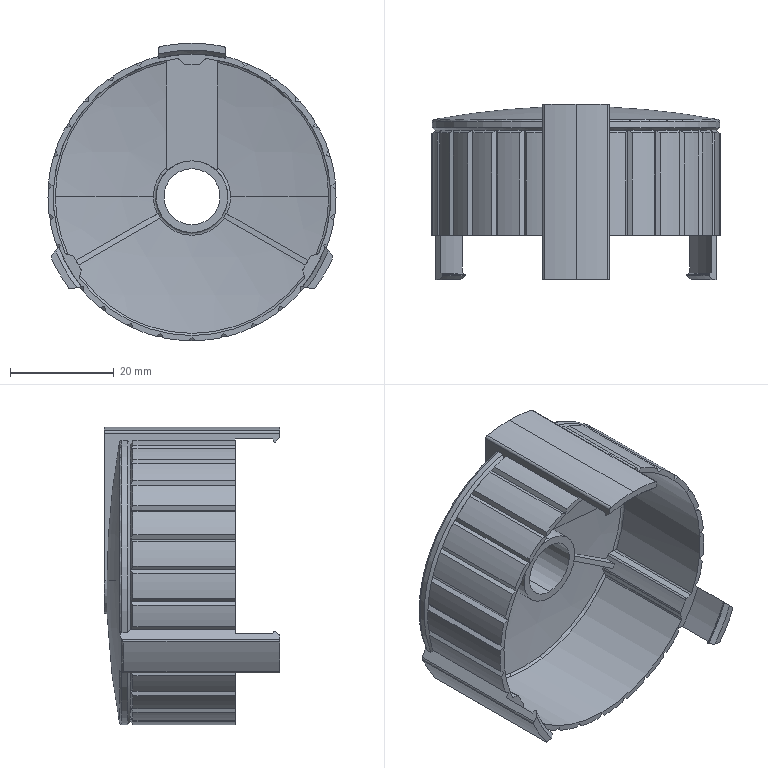Part | STEP file | PN_0053 | 1 solid | 206 faces | box 55.4 x 33.7 x 57.2 mm | volume 9406 mm3 | cylinder 74 | plane 73 | cone 34 | torus 17 | sphere 8 | commonest cylinder face diameters 55.4 x27 1 x22 0.5 x6 56 x4 59 x4 51 x3